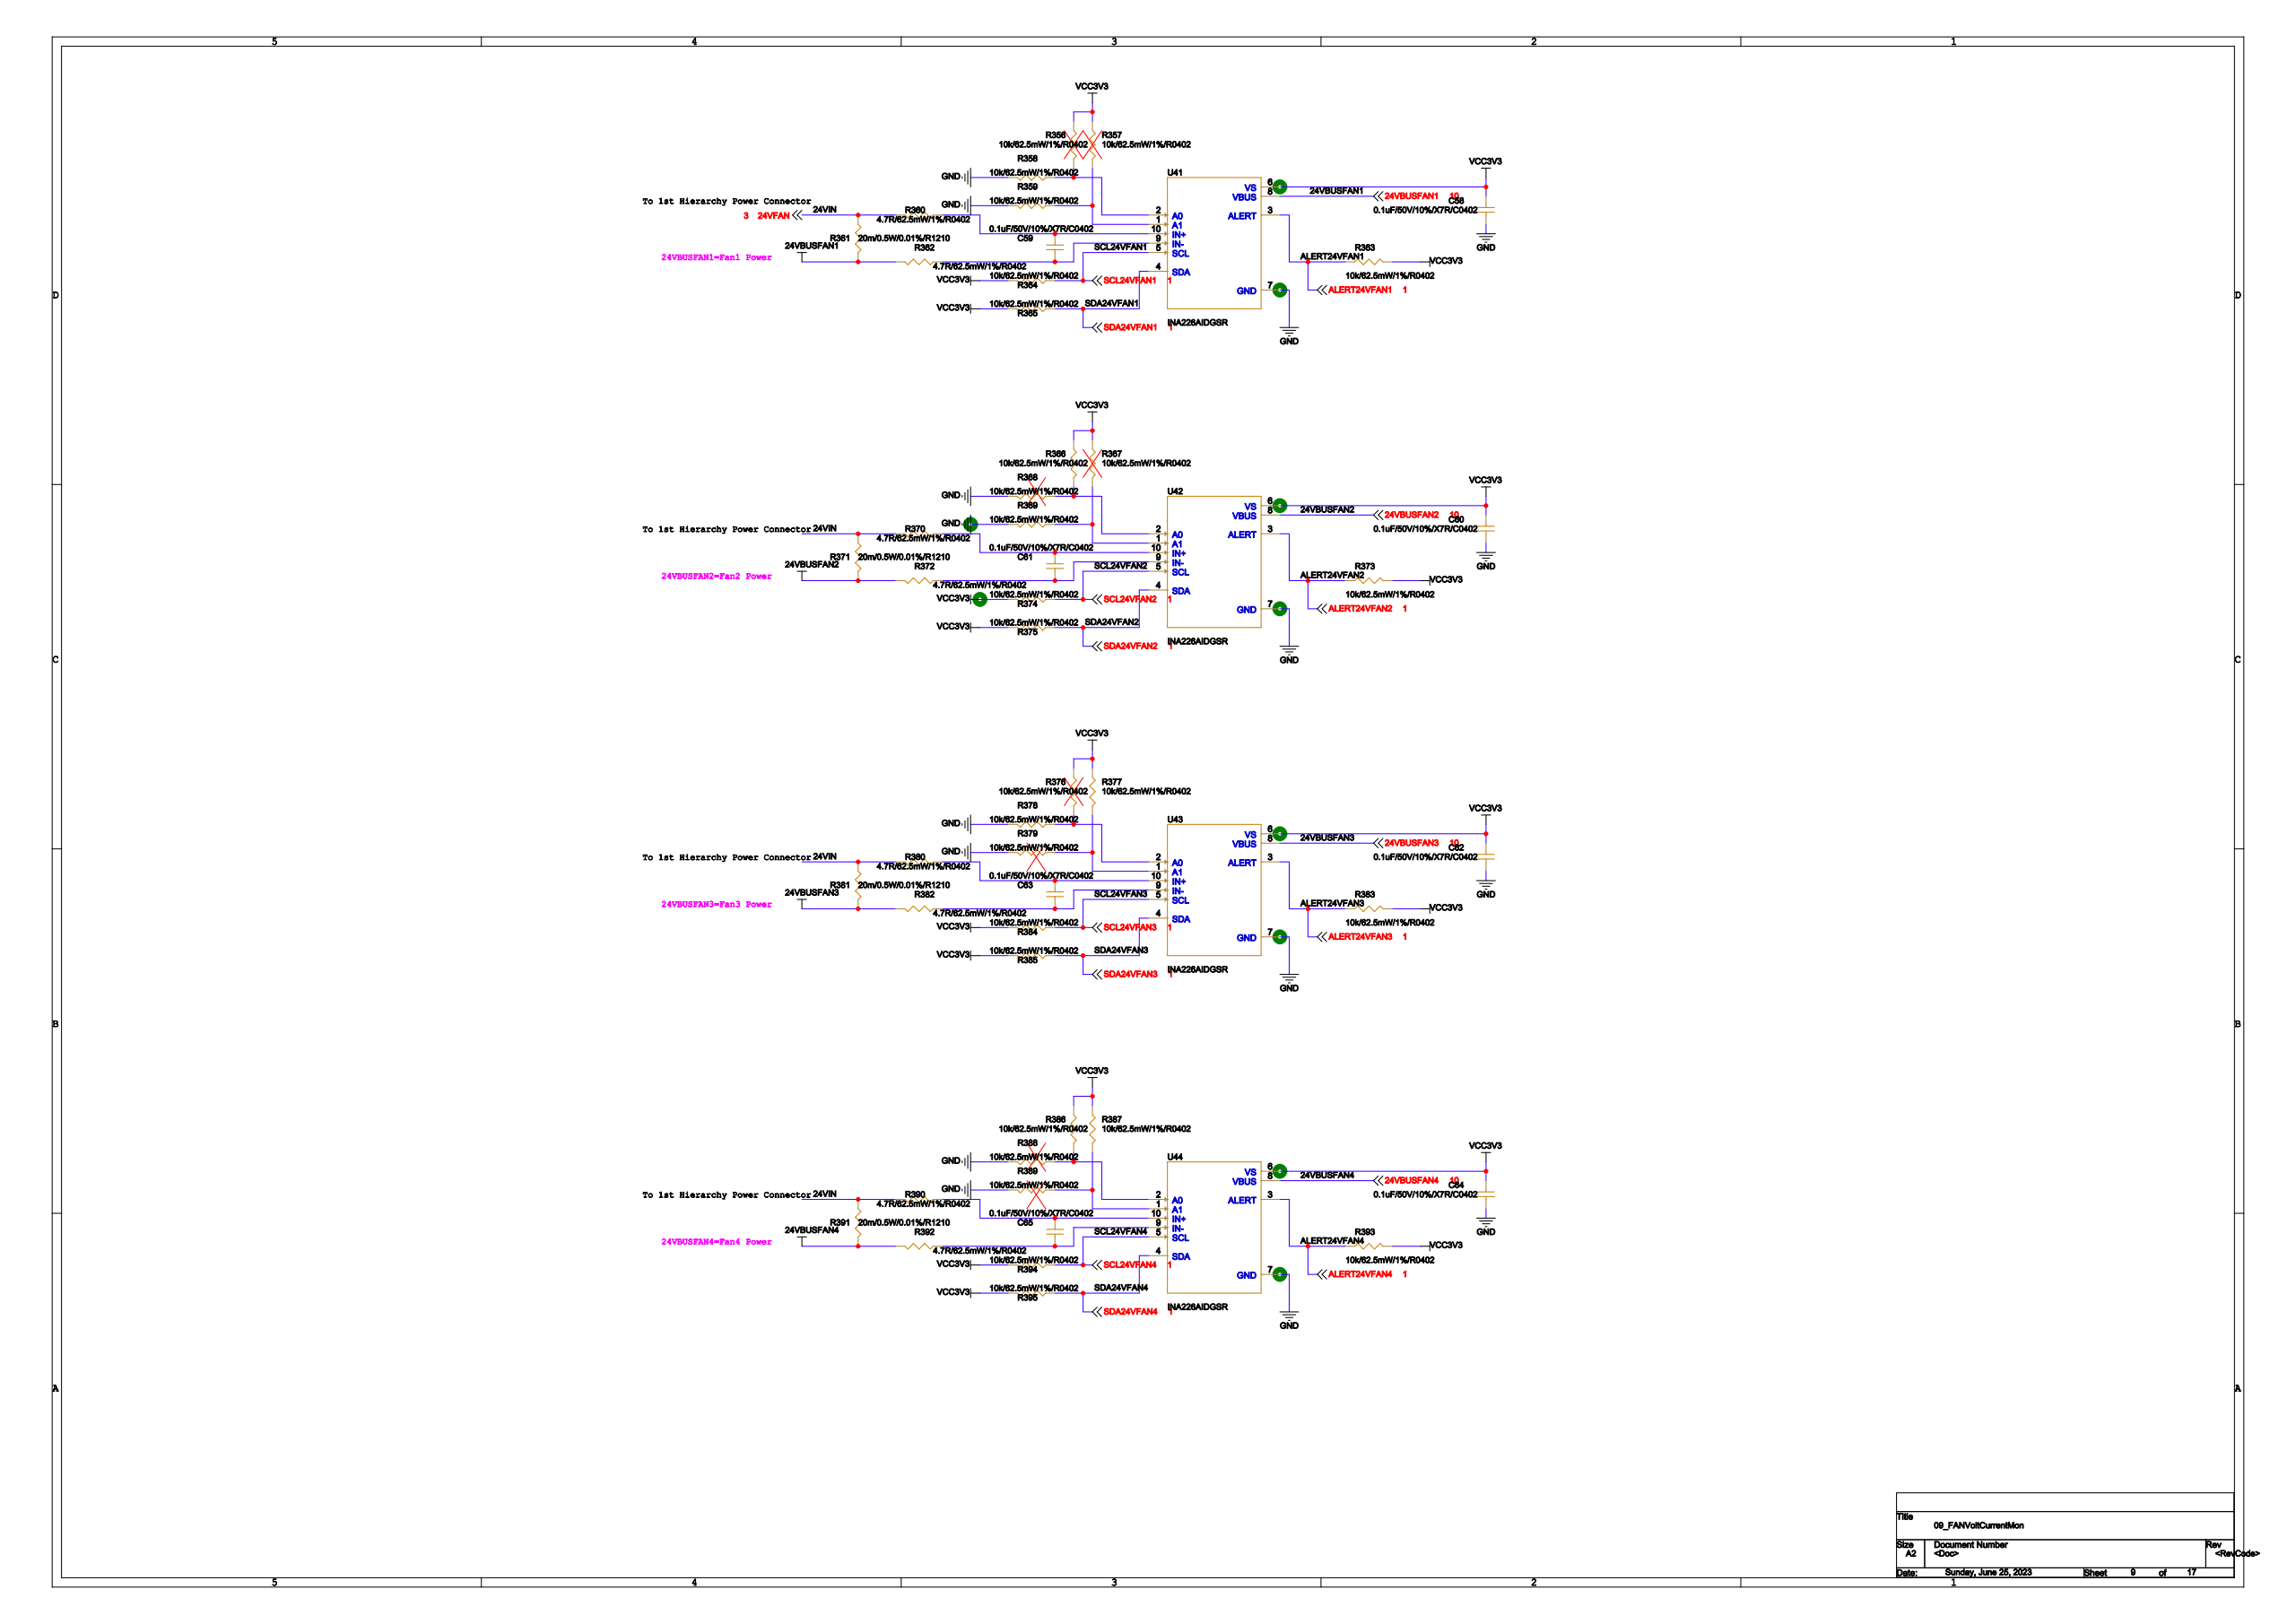Circuit board | Cadence Allegro | 2002 parts | 1538 nets | one sheet of the schematic
Parts on this sheet (reference | value | footprint):
C58 | 0.1uF/50V/10%/X7R/C0402 | 0402
C59 | 0.1uF/50V/10%/X7R/C0402 | 0402
C60 | 0.1uF/50V/10%/X7R/C0402 | 0402
C61 | 0.1uF/50V/10%/X7R/C0402 | 0402
C62 | 0.1uF/50V/10%/X7R/C0402 | 0402
C63 | 0.1uF/50V/10%/X7R/C0402 | 0402
C64 | 0.1uF/50V/10%/X7R/C0402 | 0402
C65 | 0.1uF/50V/10%/X7R/C0402 | 0402
R356 | 10k/62.5mW/1%/R0402 | 0402
R357 | 10k/62.5mW/1%/R0402 | 0402
R358 | 10k/62.5mW/1%/R0402 | 0402
R359 | 10k/62.5mW/1%/R0402 | 0402
R360 | 4.7R/62.5mW/1%/R0402 | 0402
R361 | 20m/0.5W/0.01%/R1210 | 1210
R362 | 4.7R/62.5mW/1%/R0402 | 0402
R363 | 10k/62.5mW/1%/R0402 | 0402
R364 | 10k/62.5mW/1%/R0402 | 0402
R365 | 10k/62.5mW/1%/R0402 | 0402
R366 | 10k/62.5mW/1%/R0402 | 0402
R367 | 10k/62.5mW/1%/R0402 | 0402
R368 | 10k/62.5mW/1%/R0402 | 0402
R369 | 10k/62.5mW/1%/R0402 | 0402
R370 | 4.7R/62.5mW/1%/R0402 | 0402
R371 | 20m/0.5W/0.01%/R1210 | 1210
R372 | 4.7R/62.5mW/1%/R0402 | 0402
R373 | 10k/62.5mW/1%/R0402 | 0402
R374 | 10k/62.5mW/1%/R0402 | 0402
R375 | 10k/62.5mW/1%/R0402 | 0402
R376 | 10k/62.5mW/1%/R0402 | 0402
R377 | 10k/62.5mW/1%/R0402 | 0402
R378 | 10k/62.5mW/1%/R0402 | 0402
R379 | 10k/62.5mW/1%/R0402 | 0402
R380 | 4.7R/62.5mW/1%/R0402 | 0402
R381 | 20m/0.5W/0.01%/R1210 | 1210
R382 | 4.7R/62.5mW/1%/R0402 | 0402
R383 | 10k/62.5mW/1%/R0402 | 0402
R384 | 10k/62.5mW/1%/R0402 | 0402
R385 | 10k/62.5mW/1%/R0402 | 0402
R386 | 10k/62.5mW/1%/R0402 | 0402
R387 | 10k/62.5mW/1%/R0402 | 0402
R388 | 10k/62.5mW/1%/R0402 | 0402
R389 | 10k/62.5mW/1%/R0402 | 0402
R390 | 4.7R/62.5mW/1%/R0402 | 0402
R391 | 20m/0.5W/0.01%/R1210 | 1210
R392 | 4.7R/62.5mW/1%/R0402 | 0402
R393 | 10k/62.5mW/1%/R0402 | 0402
R394 | 10k/62.5mW/1%/R0402 | 0402
R395 | 10k/62.5mW/1%/R0402 | 0402
U41 | INA226AIDGSR | SOP50P490X110-10N
U42 | INA226AIDGSR | SOP50P490X110-10N
U43 | INA226AIDGSR | SOP50P490X110-10N
U44 | INA226AIDGSR | SOP50P490X110-10N
Nets of these parts (net: part-pin ...):
3.3V: C58-1 C60-1 C62-1 C64-1 R356-1 R357-1 R363-2 R364-2 R365-2 R366-1 R367-1 R373-2 R374-2 R375-2 R376-1 R377-1 R383-2 R384-2 R385-2 R386-1 R387-1 R393-2 R394-2 R395-2 U41-6 U42-6 U43-6 U44-6
AGND: C58-2 C60-2 C62-2 C64-2 R358-2 R359-2 R368-2 R369-2 R378-2 R379-2 R388-2 R389-2 U41-7 U42-7 U43-7 U44-7
SCL24VFAN1: R364-1 U41-5
SDA24VFAN1: R365-1 U41-4
ALERT24VFAN1: R363-1 U41-3
SCL24VFAN2: R374-1 U42-5
SDA24VFAN2: R375-1 U42-4
ALERT24VFAN2: R373-1 U42-3
SCL24VFAN3: R384-1 U43-5
SDA24VFAN3: R385-1 U43-4
ALERT24VFAN3: R383-1 U43-3
ALERT24VFAN4: R393-1 U44-3
SCL24VFAN4: R394-1 U44-5
SDA24VFAN4: R395-1 U44-4
24VFAN: R360-2 R361-1 R370-2 R371-1 R380-2 R381-1 R390-2 R391-1
24VBUSFAN1: R361-2 R362-2 U41-8
24VBUSFAN4: R391-2 R392-2 U44-8
24VBUSFAN2: R371-2 R372-2 U42-8
24VBUSFAN3: R381-2 R382-2 U43-8
N23136700: C59-1 R360-1 U41-10
N23136726: C59-2 R362-1 U41-9
N23189446: C61-1 R370-1 U42-10
N23189612: C61-2 R372-1 U42-9
N23190079: C63-1 R380-1 U43-10
N23190245: C63-2 R382-1 U43-9
N23190745: C65-1 R390-1 U44-10
N23190911: C65-2 R392-1 U44-9
N23136475: R356-2 R358-1 U41-2
N23136485: R357-2 R359-1 U41-1
N23189541: R366-2 R368-1 U42-2
N23189547: R367-2 R369-1 U42-1
N23190174: R376-2 R378-1 U43-2
N23190180: R377-2 R379-1 U43-1
N23190840: R386-2 R388-1 U44-2
N23190846: R387-2 R389-1 U44-1